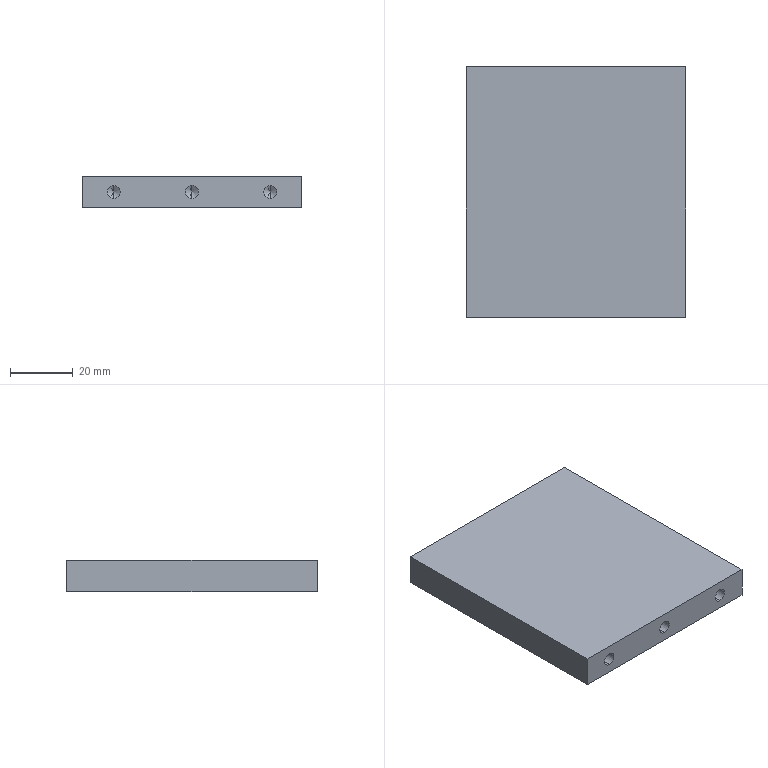Part | STEP file | C06 | 1 solid | 30 faces | box 70 x 80 x 10 mm | volume 54934 mm3 | cylinder 12 | cone 12 | plane 6 | commonest cylinder face diameters 4.2 x12